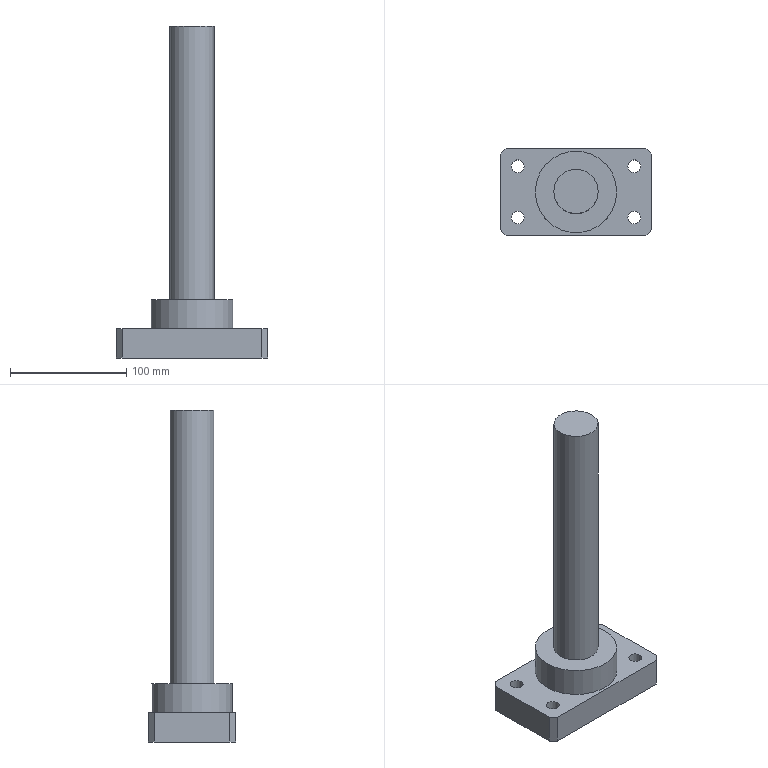Part | NX | features solid 2 | 1 solid | 18 faces | box 130 x 75 x 285 mm | volume 595725 mm3 | plane 12 | cylinder 6 | commonest cylinder face diameters 11 x4 38 x1 70 x1
STEP:
#1=CARTESIAN_POINT('',(-560.,-220.,125.));
#2=VERTEX_POINT('',#1);
#3=CARTESIAN_POINT('',(-595.,-220.,125.));
#4=DIRECTION('',(0.,0.,1.));
#5=DIRECTION('',(1.,0.,0.));
#6=AXIS2_PLACEMENT_3D('',#3,#4,#5);
#7=CIRCLE('',#6,35.);
#8=EDGE_CURVE('',#2,#2,#7,.T.);
#9=ORIENTED_EDGE('',*,*,#8,.T.);
#10=EDGE_LOOP('',(#9));
#11=FACE_BOUND('',#10,.T.);
#12=CARTESIAN_POINT('',(-576.,-220.,125.));
#13=VERTEX_POINT('',#12);
#14=CARTESIAN_POINT('',(-595.,-220.,125.));
#15=DIRECTION('',(0.,0.,1.));
#16=DIRECTION('',(1.,0.,0.));
#17=AXIS2_PLACEMENT_3D('',#14,#15,#16);
#18=CIRCLE('',#17,19.);
#19=EDGE_CURVE('',#13,#13,#18,.F.);
#20=ORIENTED_EDGE('',*,*,#19,.T.);
#21=EDGE_LOOP('',(#20));
#22=FACE_BOUND('',#21,.T.);
#23=CARTESIAN_POINT('',(-595.,-220.,125.));
#24=DIRECTION('',(0.,0.,1.));
#25=DIRECTION('',(1.,0.,0.));
#26=AXIS2_PLACEMENT_3D('',#23,#24,#25);
#27=PLANE('',#26);
#28=ADVANCED_FACE('',(#11,#22),#27,.T.);
#29=CARTESIAN_POINT('',(-639.5,-242.,100.));
#30=VERTEX_POINT('',#29);
#31=CARTESIAN_POINT('',(-645.,-242.,100.));
#32=DIRECTION('',(0.,0.,-1.));
#33=DIRECTION('',(1.,0.,0.));
#34=AXIS2_PLACEMENT_3D('',#31,#32,#33);
#35=CIRCLE('',#34,5.5);
#36=EDGE_CURVE('',#30,#30,#35,.T.);
#37=ORIENTED_EDGE('',*,*,#36,.T.);
#38=EDGE_LOOP('',(#37));
#39=FACE_BOUND('',#38,.T.);
#40=CARTESIAN_POINT('',(-639.5,-198.,100.));
#41=VERTEX_POINT('',#40);
#42=CARTESIAN_POINT('',(-645.,-198.,100.));
#43=DIRECTION('',(0.,0.,1.));
#44=DIRECTION('',(1.,0.,0.));
#45=AXIS2_PLACEMENT_3D('',#42,#43,#44);
#46=CIRCLE('',#45,5.5);
#47=EDGE_CURVE('',#41,#41,#46,.T.);
#48=ORIENTED_EDGE('',*,*,#47,.F.);
#49=EDGE_LOOP('',(#48));
#50=FACE_BOUND('',#49,.T.);
#51=CARTESIAN_POINT('',(-539.5,-198.,100.));
#52=VERTEX_POINT('',#51);
#53=CARTESIAN_POINT('',(-545.,-198.,100.));
#54=DIRECTION('',(0.,0.,1.));
#55=DIRECTION('',(1.,0.,0.));
#56=AXIS2_PLACEMENT_3D('',#53,#54,#55);
#57=CIRCLE('',#56,5.5);
#58=EDGE_CURVE('',#52,#52,#57,.T.);
#59=ORIENTED_EDGE('',*,*,#58,.F.);
#60=EDGE_LOOP('',(#59));
#61=FACE_BOUND('',#60,.T.);
#62=CARTESIAN_POINT('',(-655.,-182.5,100.));
#63=VERTEX_POINT('',#62);
#64=CARTESIAN_POINT('',(-660.,-187.5,100.));
#65=VERTEX_POINT('',#64);
#66=CARTESIAN_POINT('',(-655.,-182.5,100.));
#67=DIRECTION('',(-0.7071,-0.7071,0.));
#68=VECTOR('',#67,1000.);
#69=LINE('',#66,#68);
#70=EDGE_CURVE('',#63,#65,#69,.T.);
#71=ORIENTED_EDGE('',*,*,#70,.T.);
#72=CARTESIAN_POINT('',(-660.,-252.5,100.));
#73=VERTEX_POINT('',#72);
#74=CARTESIAN_POINT('',(-660.,-187.5,100.));
#75=DIRECTION('',(0.,-1.,0.));
#76=VECTOR('',#75,1000.);
#77=LINE('',#74,#76);
#78=EDGE_CURVE('',#65,#73,#77,.T.);
#79=ORIENTED_EDGE('',*,*,#78,.T.);
#80=CARTESIAN_POINT('',(-655.,-257.5,100.));
#81=VERTEX_POINT('',#80);
#82=CARTESIAN_POINT('',(-660.,-252.5,100.));
#83=DIRECTION('',(0.7071,-0.7071,0.));
#84=VECTOR('',#83,1000.);
#85=LINE('',#82,#84);
#86=EDGE_CURVE('',#73,#81,#85,.T.);
#87=ORIENTED_EDGE('',*,*,#86,.T.);
#88=CARTESIAN_POINT('',(-535.,-257.5,100.));
#89=VERTEX_POINT('',#88);
#90=CARTESIAN_POINT('',(-655.,-257.5,100.));
#91=DIRECTION('',(1.,0.,0.));
#92=VECTOR('',#91,1000.);
#93=LINE('',#90,#92);
#94=EDGE_CURVE('',#81,#89,#93,.T.);
#95=ORIENTED_EDGE('',*,*,#94,.T.);
#96=CARTESIAN_POINT('',(-530.,-252.5,100.));
#97=VERTEX_POINT('',#96);
#98=CARTESIAN_POINT('',(-535.,-257.5,100.));
#99=DIRECTION('',(0.7071,0.7071,0.));
#100=VECTOR('',#99,1000.);
#101=LINE('',#98,#100);
#102=EDGE_CURVE('',#89,#97,#101,.T.);
#103=ORIENTED_EDGE('',*,*,#102,.T.);
#104=CARTESIAN_POINT('',(-530.,-187.5,100.));
#105=VERTEX_POINT('',#104);
#106=CARTESIAN_POINT('',(-530.,-252.5,100.));
#107=DIRECTION('',(0.,1.,0.));
#108=VECTOR('',#107,1000.);
#109=LINE('',#106,#108);
#110=EDGE_CURVE('',#97,#105,#109,.T.);
#111=ORIENTED_EDGE('',*,*,#110,.T.);
#112=CARTESIAN_POINT('',(-535.,-182.5,100.));
#113=VERTEX_POINT('',#112);
#114=CARTESIAN_POINT('',(-530.,-187.5,100.));
#115=DIRECTION('',(-0.7071,0.7071,0.));
#116=VECTOR('',#115,1000.);
#117=LINE('',#114,#116);
#118=EDGE_CURVE('',#105,#113,#117,.T.);
#119=ORIENTED_EDGE('',*,*,#118,.T.);
#120=CARTESIAN_POINT('',(-535.,-182.5,100.));
#121=DIRECTION('',(-1.,0.,0.));
#122=VECTOR('',#121,1000.);
#123=LINE('',#120,#122);
#124=EDGE_CURVE('',#113,#63,#123,.T.);
#125=ORIENTED_EDGE('',*,*,#124,.T.);
#126=EDGE_LOOP('',(#71,#79,#87,#95,#103,#111,#119,#125));
#127=FACE_BOUND('',#126,.T.);
#128=CARTESIAN_POINT('',(-539.5,-242.,100.));
#129=VERTEX_POINT('',#128);
#130=CARTESIAN_POINT('',(-545.,-242.,100.));
#131=DIRECTION('',(0.,0.,-1.));
#132=DIRECTION('',(1.,0.,0.));
#133=AXIS2_PLACEMENT_3D('',#130,#131,#132);
#134=CIRCLE('',#133,5.5);
#135=EDGE_CURVE('',#129,#129,#134,.T.);
#136=ORIENTED_EDGE('',*,*,#135,.T.);
#137=EDGE_LOOP('',(#136));
#138=FACE_BOUND('',#137,.T.);
#139=CARTESIAN_POINT('',(-630.,-220.,100.));
#140=VERTEX_POINT('',#139);
#141=CARTESIAN_POINT('',(-595.,-220.,100.));
#142=DIRECTION('',(0.,0.,-1.));
#143=DIRECTION('',(-1.,0.,0.));
#144=AXIS2_PLACEMENT_3D('',#141,#142,#143);
#145=CIRCLE('',#144,35.);
#146=EDGE_CURVE('',#140,#140,#145,.F.);
#147=ORIENTED_EDGE('',*,*,#146,.F.);
#148=EDGE_LOOP('',(#147));
#149=FACE_BOUND('',#148,.T.);
#150=CARTESIAN_POINT('',(-595.,-122.5,100.));
#151=DIRECTION('',(0.,0.,-1.));
#152=DIRECTION('',(-1.,0.,0.));
#153=AXIS2_PLACEMENT_3D('',#150,#151,#152);
#154=PLANE('',#153);
#155=ADVANCED_FACE('',(#39,#50,#61,#127,#138,#149),#154,.F.);
#156=CARTESIAN_POINT('',(-655.,-182.5,75.));
#157=VERTEX_POINT('',#156);
#158=CARTESIAN_POINT('',(-660.,-187.5,75.));
#159=VERTEX_POINT('',#158);
#160=CARTESIAN_POINT('',(-655.,-182.5,75.));
#161=DIRECTION('',(-0.7071,-0.7071,0.));
#162=VECTOR('',#161,1000.);
#163=LINE('',#160,#162);
#164=EDGE_CURVE('',#157,#159,#163,.T.);
#165=ORIENTED_EDGE('',*,*,#164,.T.);
#166=CARTESIAN_POINT('',(-660.,-187.5,100.));
#167=DIRECTION('',(0.,0.,-1.));
#168=VECTOR('',#167,1000.);
#169=LINE('',#166,#168);
#170=EDGE_CURVE('',#65,#159,#169,.T.);
#171=ORIENTED_EDGE('',*,*,#170,.F.);
#172=ORIENTED_EDGE('',*,*,#70,.F.);
#173=CARTESIAN_POINT('',(-655.,-182.5,100.));
#174=DIRECTION('',(0.,0.,-1.));
#175=VECTOR('',#174,1000.);
#176=LINE('',#173,#175);
#177=EDGE_CURVE('',#63,#157,#176,.T.);
#178=ORIENTED_EDGE('',*,*,#177,.T.);
#179=EDGE_LOOP('',(#165,#171,#172,#178));
#180=FACE_BOUND('',#179,.T.);
#181=CARTESIAN_POINT('',(-655.,-182.5,100.));
#182=DIRECTION('',(0.7071,-0.7071,0.));
#183=DIRECTION('',(0.7071,0.7071,0.));
#184=AXIS2_PLACEMENT_3D('',#181,#182,#183);
#185=PLANE('',#184);
#186=ADVANCED_FACE('',(#180),#185,.F.);
#187=CARTESIAN_POINT('',(-660.,-252.5,75.));
#188=VERTEX_POINT('',#187);
#189=CARTESIAN_POINT('',(-660.,-187.5,75.));
#190=DIRECTION('',(0.,-1.,0.));
#191=VECTOR('',#190,1000.);
#192=LINE('',#189,#191);
#193=EDGE_CURVE('',#159,#188,#192,.T.);
#194=ORIENTED_EDGE('',*,*,#193,.T.);
#195=CARTESIAN_POINT('',(-660.,-252.5,100.));
#196=DIRECTION('',(0.,0.,-1.));
#197=VECTOR('',#196,1000.);
#198=LINE('',#195,#197);
#199=EDGE_CURVE('',#73,#188,#198,.T.);
#200=ORIENTED_EDGE('',*,*,#199,.F.);
#201=ORIENTED_EDGE('',*,*,#78,.F.);
#202=ORIENTED_EDGE('',*,*,#170,.T.);
#203=EDGE_LOOP('',(#194,#200,#201,#202));
#204=FACE_BOUND('',#203,.T.);
#205=CARTESIAN_POINT('',(-660.,-187.5,100.));
#206=DIRECTION('',(1.,0.,0.));
#207=DIRECTION('',(0.,1.,0.));
#208=AXIS2_PLACEMENT_3D('',#205,#206,#207);
#209=PLANE('',#208);
#210=ADVANCED_FACE('',(#204),#209,.F.);
#211=CARTESIAN_POINT('',(-655.,-257.5,75.));
#212=VERTEX_POINT('',#211);
#213=CARTESIAN_POINT('',(-660.,-252.5,75.));
#214=DIRECTION('',(0.7071,-0.7071,0.));
#215=VECTOR('',#214,1000.);
#216=LINE('',#213,#215);
#217=EDGE_CURVE('',#188,#212,#216,.T.);
#218=ORIENTED_EDGE('',*,*,#217,.T.);
#219=CARTESIAN_POINT('',(-655.,-257.5,100.));
#220=DIRECTION('',(0.,0.,-1.));
#221=VECTOR('',#220,1000.);
#222=LINE('',#219,#221);
#223=EDGE_CURVE('',#81,#212,#222,.T.);
#224=ORIENTED_EDGE('',*,*,#223,.F.);
#225=ORIENTED_EDGE('',*,*,#86,.F.);
#226=ORIENTED_EDGE('',*,*,#199,.T.);
#227=EDGE_LOOP('',(#218,#224,#225,#226));
#228=FACE_BOUND('',#227,.T.);
#229=CARTESIAN_POINT('',(-660.,-252.5,100.));
#230=DIRECTION('',(0.7071,0.7071,0.));
#231=DIRECTION('',(-0.7071,0.7071,0.));
#232=AXIS2_PLACEMENT_3D('',#229,#230,#231);
#233=PLANE('',#232);
#234=ADVANCED_FACE('',(#228),#233,.F.);
#235=CARTESIAN_POINT('',(-535.,-257.5,75.));
#236=VERTEX_POINT('',#235);
#237=CARTESIAN_POINT('',(-655.,-257.5,75.));
#238=DIRECTION('',(1.,0.,0.));
#239=VECTOR('',#238,1000.);
#240=LINE('',#237,#239);
#241=EDGE_CURVE('',#212,#236,#240,.T.);
#242=ORIENTED_EDGE('',*,*,#241,.T.);
#243=CARTESIAN_POINT('',(-535.,-257.5,100.));
#244=DIRECTION('',(0.,0.,-1.));
#245=VECTOR('',#244,1000.);
#246=LINE('',#243,#245);
#247=EDGE_CURVE('',#89,#236,#246,.T.);
#248=ORIENTED_EDGE('',*,*,#247,.F.);
#249=ORIENTED_EDGE('',*,*,#94,.F.);
#250=ORIENTED_EDGE('',*,*,#223,.T.);
#251=EDGE_LOOP('',(#242,#248,#249,#250));
#252=FACE_BOUND('',#251,.T.);
#253=CARTESIAN_POINT('',(-655.,-257.5,100.));
#254=DIRECTION('',(0.,1.,0.));
#255=DIRECTION('',(-1.,0.,0.));
#256=AXIS2_PLACEMENT_3D('',#253,#254,#255);
#257=PLANE('',#256);
#258=ADVANCED_FACE('',(#252),#257,.F.);
#259=CARTESIAN_POINT('',(-530.,-252.5,75.));
#260=VERTEX_POINT('',#259);
#261=CARTESIAN_POINT('',(-535.,-257.5,75.));
#262=DIRECTION('',(0.7071,0.7071,0.));
#263=VECTOR('',#262,1000.);
#264=LINE('',#261,#263);
#265=EDGE_CURVE('',#236,#260,#264,.T.);
#266=ORIENTED_EDGE('',*,*,#265,.T.);
#267=CARTESIAN_POINT('',(-530.,-252.5,100.));
#268=DIRECTION('',(0.,0.,-1.));
#269=VECTOR('',#268,1000.);
#270=LINE('',#267,#269);
#271=EDGE_CURVE('',#97,#260,#270,.T.);
#272=ORIENTED_EDGE('',*,*,#271,.F.);
#273=ORIENTED_EDGE('',*,*,#102,.F.);
#274=ORIENTED_EDGE('',*,*,#247,.T.);
#275=EDGE_LOOP('',(#266,#272,#273,#274));
#276=FACE_BOUND('',#275,.T.);
#277=CARTESIAN_POINT('',(-535.,-257.5,100.));
#278=DIRECTION('',(-0.7071,0.7071,0.));
#279=DIRECTION('',(-0.7071,-0.7071,0.));
#280=AXIS2_PLACEMENT_3D('',#277,#278,#279);
#281=PLANE('',#280);
#282=ADVANCED_FACE('',(#276),#281,.F.);
#283=CARTESIAN_POINT('',(-530.,-187.5,75.));
#284=VERTEX_POINT('',#283);
#285=CARTESIAN_POINT('',(-530.,-252.5,75.));
#286=DIRECTION('',(0.,1.,0.));
#287=VECTOR('',#286,1000.);
#288=LINE('',#285,#287);
#289=EDGE_CURVE('',#260,#284,#288,.T.);
#290=ORIENTED_EDGE('',*,*,#289,.T.);
#291=CARTESIAN_POINT('',(-530.,-187.5,100.));
#292=DIRECTION('',(0.,0.,-1.));
#293=VECTOR('',#292,1000.);
#294=LINE('',#291,#293);
#295=EDGE_CURVE('',#105,#284,#294,.T.);
#296=ORIENTED_EDGE('',*,*,#295,.F.);
#297=ORIENTED_EDGE('',*,*,#110,.F.);
#298=ORIENTED_EDGE('',*,*,#271,.T.);
#299=EDGE_LOOP('',(#290,#296,#297,#298));
#300=FACE_BOUND('',#299,.T.);
#301=CARTESIAN_POINT('',(-530.,-252.5,100.));
#302=DIRECTION('',(-1.,0.,0.));
#303=DIRECTION('',(0.,0.,1.));
#304=AXIS2_PLACEMENT_3D('',#301,#302,#303);
#305=PLANE('',#304);
#306=ADVANCED_FACE('',(#300),#305,.F.);
#307=CARTESIAN_POINT('',(-535.,-182.5,75.));
#308=VERTEX_POINT('',#307);
#309=CARTESIAN_POINT('',(-530.,-187.5,75.));
#310=DIRECTION('',(-0.7071,0.7071,0.));
#311=VECTOR('',#310,1000.);
#312=LINE('',#309,#311);
#313=EDGE_CURVE('',#284,#308,#312,.T.);
#314=ORIENTED_EDGE('',*,*,#313,.T.);
#315=CARTESIAN_POINT('',(-535.,-182.5,100.));
#316=DIRECTION('',(0.,0.,-1.));
#317=VECTOR('',#316,1000.);
#318=LINE('',#315,#317);
#319=EDGE_CURVE('',#113,#308,#318,.T.);
#320=ORIENTED_EDGE('',*,*,#319,.F.);
#321=ORIENTED_EDGE('',*,*,#118,.F.);
#322=ORIENTED_EDGE('',*,*,#295,.T.);
#323=EDGE_LOOP('',(#314,#320,#321,#322));
#324=FACE_BOUND('',#323,.T.);
#325=CARTESIAN_POINT('',(-530.,-187.5,100.));
#326=DIRECTION('',(-0.7071,-0.7071,0.));
#327=DIRECTION('',(0.7071,-0.7071,0.));
#328=AXIS2_PLACEMENT_3D('',#325,#326,#327);
#329=PLANE('',#328);
#330=ADVANCED_FACE('',(#324),#329,.F.);
#331=ORIENTED_EDGE('',*,*,#47,.T.);
#332=EDGE_LOOP('',(#331));
#333=FACE_BOUND('',#332,.T.);
#334=CARTESIAN_POINT('',(-639.5,-198.,75.));
#335=VERTEX_POINT('',#334);
#336=CARTESIAN_POINT('',(-645.,-198.,75.));
#337=DIRECTION('',(0.,0.,1.));
#338=DIRECTION('',(1.,0.,0.));
#339=AXIS2_PLACEMENT_3D('',#336,#337,#338);
#340=CIRCLE('',#339,5.5);
#341=EDGE_CURVE('',#335,#335,#340,.T.);
#342=ORIENTED_EDGE('',*,*,#341,.F.);
#343=EDGE_LOOP('',(#342));
#344=FACE_BOUND('',#343,.T.);
#345=CARTESIAN_POINT('',(-645.,-198.,100.));
#346=DIRECTION('',(0.,0.,-1.));
#347=DIRECTION('',(-1.,0.,0.));
#348=AXIS2_PLACEMENT_3D('',#345,#346,#347);
#349=CYLINDRICAL_SURFACE('',#348,5.5);
#350=ADVANCED_FACE('',(#333,#344),#349,.F.);
#351=ORIENTED_EDGE('',*,*,#58,.T.);
#352=EDGE_LOOP('',(#351));
#353=FACE_BOUND('',#352,.T.);
#354=CARTESIAN_POINT('',(-539.5,-198.,75.));
#355=VERTEX_POINT('',#354);
#356=CARTESIAN_POINT('',(-545.,-198.,75.));
#357=DIRECTION('',(0.,0.,1.));
#358=DIRECTION('',(1.,0.,0.));
#359=AXIS2_PLACEMENT_3D('',#356,#357,#358);
#360=CIRCLE('',#359,5.5);
#361=EDGE_CURVE('',#355,#355,#360,.T.);
#362=ORIENTED_EDGE('',*,*,#361,.F.);
#363=EDGE_LOOP('',(#362));
#364=FACE_BOUND('',#363,.T.);
#365=CARTESIAN_POINT('',(-545.,-198.,100.));
#366=DIRECTION('',(0.,0.,-1.));
#367=DIRECTION('',(-1.,0.,0.));
#368=AXIS2_PLACEMENT_3D('',#365,#366,#367);
#369=CYLINDRICAL_SURFACE('',#368,5.5);
#370=ADVANCED_FACE('',(#353,#364),#369,.F.);
#371=CARTESIAN_POINT('',(-535.,-182.5,75.));
#372=DIRECTION('',(-1.,0.,0.));
#373=VECTOR('',#372,1000.);
#374=LINE('',#371,#373);
#375=EDGE_CURVE('',#308,#157,#374,.T.);
#376=ORIENTED_EDGE('',*,*,#375,.T.);
#377=ORIENTED_EDGE('',*,*,#177,.F.);
#378=ORIENTED_EDGE('',*,*,#124,.F.);
#379=ORIENTED_EDGE('',*,*,#319,.T.);
#380=EDGE_LOOP('',(#376,#377,#378,#379));
#381=FACE_BOUND('',#380,.T.);
#382=CARTESIAN_POINT('',(-535.,-182.5,100.));
#383=DIRECTION('',(0.,-1.,0.));
#384=DIRECTION('',(0.,0.,-1.));
#385=AXIS2_PLACEMENT_3D('',#382,#383,#384);
#386=PLANE('',#385);
#387=ADVANCED_FACE('',(#381),#386,.F.);
#388=ORIENTED_EDGE('',*,*,#135,.F.);
#389=EDGE_LOOP('',(#388));
#390=FACE_BOUND('',#389,.T.);
#391=CARTESIAN_POINT('',(-539.5,-242.,75.));
#392=VERTEX_POINT('',#391);
#393=CARTESIAN_POINT('',(-545.,-242.,75.));
#394=DIRECTION('',(0.,0.,-1.));
#395=DIRECTION('',(1.,0.,0.));
#396=AXIS2_PLACEMENT_3D('',#393,#394,#395);
#397=CIRCLE('',#396,5.5);
#398=EDGE_CURVE('',#392,#392,#397,.T.);
#399=ORIENTED_EDGE('',*,*,#398,.T.);
#400=EDGE_LOOP('',(#399));
#401=FACE_BOUND('',#400,.T.);
#402=CARTESIAN_POINT('',(-545.,-242.,100.));
#403=DIRECTION('',(0.,0.,-1.));
#404=DIRECTION('',(-1.,0.,0.));
#405=AXIS2_PLACEMENT_3D('',#402,#403,#404);
#406=CYLINDRICAL_SURFACE('',#405,5.5);
#407=ADVANCED_FACE('',(#390,#401),#406,.F.);
#408=ORIENTED_EDGE('',*,*,#36,.F.);
#409=EDGE_LOOP('',(#408));
#410=FACE_BOUND('',#409,.T.);
#411=CARTESIAN_POINT('',(-639.5,-242.,75.));
#412=VERTEX_POINT('',#411);
#413=CARTESIAN_POINT('',(-645.,-242.,75.));
#414=DIRECTION('',(0.,0.,-1.));
#415=DIRECTION('',(1.,0.,0.));
#416=AXIS2_PLACEMENT_3D('',#413,#414,#415);
#417=CIRCLE('',#416,5.5);
#418=EDGE_CURVE('',#412,#412,#417,.T.);
#419=ORIENTED_EDGE('',*,*,#418,.T.);
#420=EDGE_LOOP('',(#419));
#421=FACE_BOUND('',#420,.T.);
#422=CARTESIAN_POINT('',(-645.,-242.,100.));
#423=DIRECTION('',(0.,0.,-1.));
#424=DIRECTION('',(-1.,0.,0.));
#425=AXIS2_PLACEMENT_3D('',#422,#423,#424);
#426=CYLINDRICAL_SURFACE('',#425,5.5);
#427=ADVANCED_FACE('',(#410,#421),#426,.F.);
#428=ORIENTED_EDGE('',*,*,#398,.F.);
#429=EDGE_LOOP('',(#428));
#430=FACE_BOUND('',#429,.T.);
#431=ORIENTED_EDGE('',*,*,#164,.F.);
#432=ORIENTED_EDGE('',*,*,#375,.F.);
#433=ORIENTED_EDGE('',*,*,#313,.F.);
#434=ORIENTED_EDGE('',*,*,#289,.F.);
#435=ORIENTED_EDGE('',*,*,#265,.F.);
#436=ORIENTED_EDGE('',*,*,#241,.F.);
#437=ORIENTED_EDGE('',*,*,#217,.F.);
#438=ORIENTED_EDGE('',*,*,#193,.F.);
#439=EDGE_LOOP('',(#431,#432,#433,#434,#435,#436,#437,#438));
#440=FACE_BOUND('',#439,.T.);
#441=ORIENTED_EDGE('',*,*,#361,.T.);
#442=EDGE_LOOP('',(#441));
#443=FACE_BOUND('',#442,.T.);
#444=ORIENTED_EDGE('',*,*,#341,.T.);
#445=EDGE_LOOP('',(#444));
#446=FACE_BOUND('',#445,.T.);
#447=ORIENTED_EDGE('',*,*,#418,.F.);
#448=EDGE_LOOP('',(#447));
#449=FACE_BOUND('',#448,.T.);
#450=CARTESIAN_POINT('',(-595.,-122.5,75.));
#451=DIRECTION('',(0.,0.,-1.));
#452=DIRECTION('',(-1.,0.,0.));
#453=AXIS2_PLACEMENT_3D('',#450,#451,#452);
#454=PLANE('',#453);
#455=ADVANCED_FACE('',(#430,#440,#443,#446,#449),#454,.T.);
#456=ORIENTED_EDGE('',*,*,#8,.F.);
#457=EDGE_LOOP('',(#456));
#458=FACE_BOUND('',#457,.T.);
#459=ORIENTED_EDGE('',*,*,#146,.T.);
#460=EDGE_LOOP('',(#459));
#461=FACE_BOUND('',#460,.T.);
#462=CARTESIAN_POINT('',(-595.,-220.,125.));
#463=DIRECTION('',(0.,0.,-1.));
#464=DIRECTION('',(-1.,0.,0.));
#465=AXIS2_PLACEMENT_3D('',#462,#463,#464);
#466=CYLINDRICAL_SURFACE('',#465,35.);
#467=ADVANCED_FACE('',(#458,#461),#466,.T.);
#468=ORIENTED_EDGE('',*,*,#19,.F.);
#469=EDGE_LOOP('',(#468));
#470=FACE_BOUND('',#469,.T.);
#471=CARTESIAN_POINT('',(-576.,-220.,360.));
#472=VERTEX_POINT('',#471);
#473=CARTESIAN_POINT('',(-595.,-220.,360.));
#474=DIRECTION('',(0.,0.,1.));
#475=DIRECTION('',(1.,0.,0.));
#476=AXIS2_PLACEMENT_3D('',#473,#474,#475);
#477=CIRCLE('',#476,19.);
#478=EDGE_CURVE('',#472,#472,#477,.T.);
#479=ORIENTED_EDGE('',*,*,#478,.F.);
#480=EDGE_LOOP('',(#479));
#481=FACE_BOUND('',#480,.T.);
#482=CARTESIAN_POINT('',(-595.,-220.,375.));
#483=DIRECTION('',(0.,0.,-1.));
#484=DIRECTION('',(-1.,0.,0.));
#485=AXIS2_PLACEMENT_3D('',#482,#483,#484);
#486=CYLINDRICAL_SURFACE('',#485,19.);
#487=ADVANCED_FACE('',(#470,#481),#486,.T.);
#488=ORIENTED_EDGE('',*,*,#478,.T.);
#489=EDGE_LOOP('',(#488));
#490=FACE_BOUND('',#489,.T.);
#491=CARTESIAN_POINT('',(-595.,-220.,360.));
#492=DIRECTION('',(0.,0.,1.));
#493=DIRECTION('',(1.,0.,0.));
#494=AXIS2_PLACEMENT_3D('',#491,#492,#493);
#495=PLANE('',#494);
#496=ADVANCED_FACE('',(#490),#495,.T.);
#497=CLOSED_SHELL('',(#28,#155,#186,#210,#234,#258,#282,#306,#330,#350,#370,#387,#407,#427,#455,#467,#487,#496));
#498=MANIFOLD_SOLID_BREP('',#497);
#499=(LENGTH_UNIT()NAMED_UNIT(*)SI_UNIT(.MILLI.,.METRE.));
#500=UNCERTAINTY_MEASURE_WITH_UNIT(LENGTH_MEASURE(0.00001),#499,'','');
#501=(NAMED_UNIT(*)PLANE_ANGLE_UNIT()SI_UNIT($,.RADIAN.));
#502=(NAMED_UNIT(*)SI_UNIT($,.STERADIAN.)SOLID_ANGLE_UNIT());
#503=(GEOMETRIC_REPRESENTATION_CONTEXT(3)GLOBAL_UNCERTAINTY_ASSIGNED_CONTEXT((#500))GLOBAL_UNIT_ASSIGNED_CONTEXT((#499,#501,#502))REPRESENTATION_CONTEXT('',''));
#504=ADVANCED_BREP_SHAPE_REPRESENTATION('',(#498),#503);